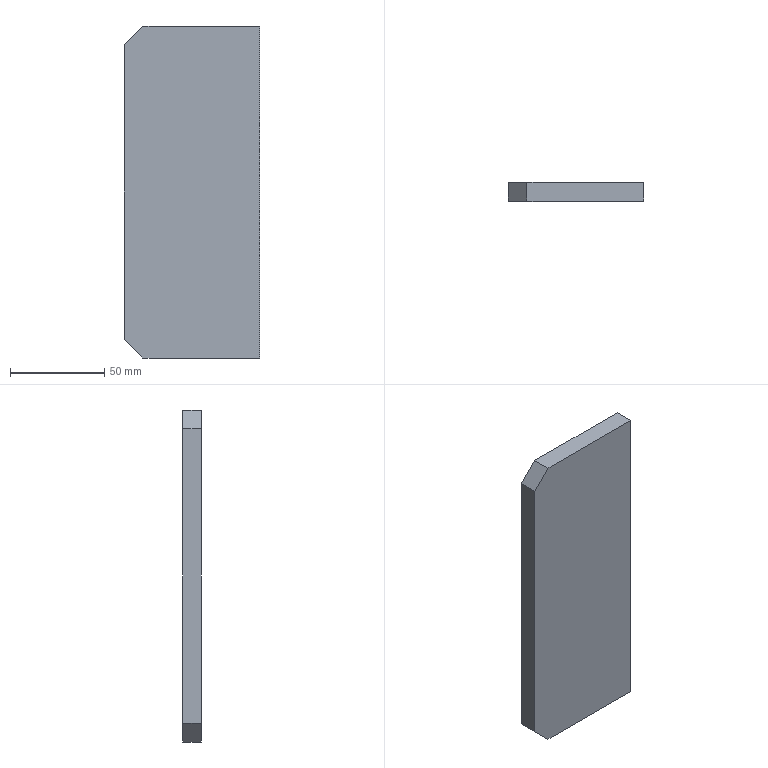Part | STEP file | 立柱填充筋Plate 200×150 | 1 solid | 8 faces | box 72 x 10 x 176 mm | volume 125720 mm3 | plane 8
STEP:
#1=CARTESIAN_POINT('',(0.,0.,0.));
#2=DIRECTION('',(0.,0.,1.));
#3=DIRECTION('',(1.,0.,0.));
#4=AXIS2_PLACEMENT_3D('',#1,#2,#3);
#5=CARTESIAN_POINT('',(72.,0.,88.));
#6=VERTEX_POINT('',#5);
#7=CARTESIAN_POINT('',(72.,0.,-88.));
#8=VERTEX_POINT('',#7);
#9=CARTESIAN_POINT('',(72.,0.,-88.));
#10=DIRECTION('',(0.,0.,-1.));
#11=VECTOR('',#10,1.);
#12=LINE('',#9,#11);
#13=CARTESIAN_POINT('',(72.,10.,-88.));
#14=DIRECTION('',(-1.,0.,0.));
#15=DIRECTION('',(0.,0.,1.));
#16=AXIS2_PLACEMENT_3D('',#13,#14,#15);
#17=PLANE('',#16);
#18=CARTESIAN_POINT('',(0.,-10.));
#19=DIRECTION('',(-1.,0.));
#20=VECTOR('',#19,1.);
#21=LINE('',#18,#20);
#22=(GEOMETRIC_REPRESENTATION_CONTEXT(2)PARAMETRIC_REPRESENTATION_CONTEXT()REPRESENTATION_CONTEXT('',''));
#23=DEFINITIONAL_REPRESENTATION('',(#21),#22);
#24=PCURVE('',#17,#23);
#25=CARTESIAN_POINT('',(0.,0.,0.));
#26=DIRECTION('',(0.,-1.,0.));
#27=DIRECTION('',(0.,0.,-1.));
#28=AXIS2_PLACEMENT_3D('',#25,#26,#27);
#29=PLANE('',#28);
#30=CARTESIAN_POINT('',(88.,72.));
#31=DIRECTION('',(1.,0.));
#32=VECTOR('',#31,1.);
#33=LINE('',#30,#32);
#34=(GEOMETRIC_REPRESENTATION_CONTEXT(2)PARAMETRIC_REPRESENTATION_CONTEXT()REPRESENTATION_CONTEXT('',''));
#35=DEFINITIONAL_REPRESENTATION('',(#33),#34);
#36=PCURVE('',#29,#35);
#37=SURFACE_CURVE('',#12,(#24,#36),.PCURVE_S1.);
#38=EDGE_CURVE('',#6,#8,#37,.T.);
#39=ORIENTED_EDGE('',*,*,#38,.T.);
#40=CARTESIAN_POINT('',(72.,10.,-88.));
#41=VERTEX_POINT('',#40);
#42=CARTESIAN_POINT('',(72.,10.,-88.));
#43=DIRECTION('',(0.,-1.,0.));
#44=VECTOR('',#43,1.);
#45=LINE('',#42,#44);
#46=CARTESIAN_POINT('',(0.,0.));
#47=DIRECTION('',(0.,-1.));
#48=VECTOR('',#47,1.);
#49=LINE('',#46,#48);
#50=(GEOMETRIC_REPRESENTATION_CONTEXT(2)PARAMETRIC_REPRESENTATION_CONTEXT()REPRESENTATION_CONTEXT('',''));
#51=DEFINITIONAL_REPRESENTATION('',(#49),#50);
#52=PCURVE('',#17,#51);
#53=CARTESIAN_POINT('',(0.,10.,-88.));
#54=DIRECTION('',(0.,0.,1.));
#55=DIRECTION('',(1.,0.,0.));
#56=AXIS2_PLACEMENT_3D('',#53,#54,#55);
#57=PLANE('',#56);
#58=CARTESIAN_POINT('',(72.,0.));
#59=DIRECTION('',(0.,-1.));
#60=VECTOR('',#59,1.);
#61=LINE('',#58,#60);
#62=(GEOMETRIC_REPRESENTATION_CONTEXT(2)PARAMETRIC_REPRESENTATION_CONTEXT()REPRESENTATION_CONTEXT('',''));
#63=DEFINITIONAL_REPRESENTATION('',(#61),#62);
#64=PCURVE('',#57,#63);
#65=SURFACE_CURVE('',#45,(#52,#64),.PCURVE_S1.);
#66=EDGE_CURVE('',#41,#8,#65,.T.);
#67=ORIENTED_EDGE('',*,*,#66,.F.);
#68=CARTESIAN_POINT('',(72.,10.,88.));
#69=VERTEX_POINT('',#68);
#70=CARTESIAN_POINT('',(72.,10.,-88.));
#71=DIRECTION('',(0.,0.,-1.));
#72=VECTOR('',#71,1.);
#73=LINE('',#70,#72);
#74=CARTESIAN_POINT('',(0.,0.));
#75=DIRECTION('',(-1.,0.));
#76=VECTOR('',#75,1.);
#77=LINE('',#74,#76);
#78=(GEOMETRIC_REPRESENTATION_CONTEXT(2)PARAMETRIC_REPRESENTATION_CONTEXT()REPRESENTATION_CONTEXT('',''));
#79=DEFINITIONAL_REPRESENTATION('',(#77),#78);
#80=PCURVE('',#17,#79);
#81=CARTESIAN_POINT('',(0.,10.,0.));
#82=DIRECTION('',(0.,-1.,0.));
#83=DIRECTION('',(0.,0.,-1.));
#84=AXIS2_PLACEMENT_3D('',#81,#82,#83);
#85=PLANE('',#84);
#86=CARTESIAN_POINT('',(88.,72.));
#87=DIRECTION('',(1.,0.));
#88=VECTOR('',#87,1.);
#89=LINE('',#86,#88);
#90=(GEOMETRIC_REPRESENTATION_CONTEXT(2)PARAMETRIC_REPRESENTATION_CONTEXT()REPRESENTATION_CONTEXT('',''));
#91=DEFINITIONAL_REPRESENTATION('',(#89),#90);
#92=PCURVE('',#85,#91);
#93=SURFACE_CURVE('',#73,(#80,#92),.PCURVE_S1.);
#94=EDGE_CURVE('',#69,#41,#93,.T.);
#95=ORIENTED_EDGE('',*,*,#94,.F.);
#96=CARTESIAN_POINT('',(72.,10.,88.));
#97=DIRECTION('',(0.,-1.,0.));
#98=VECTOR('',#97,1.);
#99=LINE('',#96,#98);
#100=CARTESIAN_POINT('',(176.,0.));
#101=DIRECTION('',(0.,-1.));
#102=VECTOR('',#101,1.);
#103=LINE('',#100,#102);
#104=(GEOMETRIC_REPRESENTATION_CONTEXT(2)PARAMETRIC_REPRESENTATION_CONTEXT()REPRESENTATION_CONTEXT('',''));
#105=DEFINITIONAL_REPRESENTATION('',(#103),#104);
#106=PCURVE('',#17,#105);
#107=CARTESIAN_POINT('',(72.,10.,88.));
#108=DIRECTION('',(0.,0.,-1.));
#109=DIRECTION('',(-1.,0.,0.));
#110=AXIS2_PLACEMENT_3D('',#107,#108,#109);
#111=PLANE('',#110);
#112=CARTESIAN_POINT('',(0.,0.));
#113=DIRECTION('',(0.,-1.));
#114=VECTOR('',#113,1.);
#115=LINE('',#112,#114);
#116=(GEOMETRIC_REPRESENTATION_CONTEXT(2)PARAMETRIC_REPRESENTATION_CONTEXT()REPRESENTATION_CONTEXT('',''));
#117=DEFINITIONAL_REPRESENTATION('',(#115),#116);
#118=PCURVE('',#111,#117);
#119=SURFACE_CURVE('',#99,(#106,#118),.PCURVE_S1.);
#120=EDGE_CURVE('',#69,#6,#119,.T.);
#121=ORIENTED_EDGE('',*,*,#120,.T.);
#122=EDGE_LOOP('',(#39,#67,#95,#121));
#123=FACE_BOUND('',#122,.T.);
#124=ADVANCED_FACE('',(#123),#17,.F.);
#125=CARTESIAN_POINT('',(10.,0.,-88.));
#126=VERTEX_POINT('',#125);
#127=CARTESIAN_POINT('',(0.,0.,-88.));
#128=DIRECTION('',(-1.,0.,0.));
#129=VECTOR('',#128,1.);
#130=LINE('',#127,#129);
#131=CARTESIAN_POINT('',(0.,-10.));
#132=DIRECTION('',(-1.,0.));
#133=VECTOR('',#132,1.);
#134=LINE('',#131,#133);
#135=(GEOMETRIC_REPRESENTATION_CONTEXT(2)PARAMETRIC_REPRESENTATION_CONTEXT()REPRESENTATION_CONTEXT('',''));
#136=DEFINITIONAL_REPRESENTATION('',(#134),#135);
#137=PCURVE('',#57,#136);
#138=CARTESIAN_POINT('',(88.,0.));
#139=DIRECTION('',(0.,-1.));
#140=VECTOR('',#139,1.);
#141=LINE('',#138,#140);
#142=(GEOMETRIC_REPRESENTATION_CONTEXT(2)PARAMETRIC_REPRESENTATION_CONTEXT()REPRESENTATION_CONTEXT('',''));
#143=DEFINITIONAL_REPRESENTATION('',(#141),#142);
#144=PCURVE('',#29,#143);
#145=SURFACE_CURVE('',#130,(#137,#144),.PCURVE_S1.);
#146=EDGE_CURVE('',#8,#126,#145,.T.);
#147=ORIENTED_EDGE('',*,*,#146,.T.);
#148=CARTESIAN_POINT('',(10.,10.,-88.));
#149=VERTEX_POINT('',#148);
#150=CARTESIAN_POINT('',(10.,10.,-88.));
#151=DIRECTION('',(0.,1.,0.));
#152=VECTOR('',#151,1.);
#153=LINE('',#150,#152);
#154=CARTESIAN_POINT('',(10.,0.));
#155=DIRECTION('',(0.,1.));
#156=VECTOR('',#155,1.);
#157=LINE('',#154,#156);
#158=(GEOMETRIC_REPRESENTATION_CONTEXT(2)PARAMETRIC_REPRESENTATION_CONTEXT()REPRESENTATION_CONTEXT('',''));
#159=DEFINITIONAL_REPRESENTATION('',(#157),#158);
#160=PCURVE('',#57,#159);
#161=CARTESIAN_POINT('',(0.,10.,-78.));
#162=DIRECTION('',(0.7071,0.,0.7071));
#163=DIRECTION('',(0.,-1.,0.));
#164=AXIS2_PLACEMENT_3D('',#161,#162,#163);
#165=PLANE('',#164);
#166=CARTESIAN_POINT('',(0.,14.142));
#167=DIRECTION('',(-1.,0.));
#168=VECTOR('',#167,1.);
#169=LINE('',#166,#168);
#170=(GEOMETRIC_REPRESENTATION_CONTEXT(2)PARAMETRIC_REPRESENTATION_CONTEXT()REPRESENTATION_CONTEXT('',''));
#171=DEFINITIONAL_REPRESENTATION('',(#169),#170);
#172=PCURVE('',#165,#171);
#173=SURFACE_CURVE('',#153,(#160,#172),.PCURVE_S1.);
#174=EDGE_CURVE('',#126,#149,#173,.T.);
#175=ORIENTED_EDGE('',*,*,#174,.T.);
#176=CARTESIAN_POINT('',(0.,10.,-88.));
#177=DIRECTION('',(-1.,0.,0.));
#178=VECTOR('',#177,1.);
#179=LINE('',#176,#178);
#180=CARTESIAN_POINT('',(0.,0.));
#181=DIRECTION('',(-1.,0.));
#182=VECTOR('',#181,1.);
#183=LINE('',#180,#182);
#184=(GEOMETRIC_REPRESENTATION_CONTEXT(2)PARAMETRIC_REPRESENTATION_CONTEXT()REPRESENTATION_CONTEXT('',''));
#185=DEFINITIONAL_REPRESENTATION('',(#183),#184);
#186=PCURVE('',#57,#185);
#187=CARTESIAN_POINT('',(88.,0.));
#188=DIRECTION('',(0.,-1.));
#189=VECTOR('',#188,1.);
#190=LINE('',#187,#189);
#191=(GEOMETRIC_REPRESENTATION_CONTEXT(2)PARAMETRIC_REPRESENTATION_CONTEXT()REPRESENTATION_CONTEXT('',''));
#192=DEFINITIONAL_REPRESENTATION('',(#190),#191);
#193=PCURVE('',#85,#192);
#194=SURFACE_CURVE('',#179,(#186,#193),.PCURVE_S1.);
#195=EDGE_CURVE('',#41,#149,#194,.T.);
#196=ORIENTED_EDGE('',*,*,#195,.F.);
#197=ORIENTED_EDGE('',*,*,#66,.T.);
#198=EDGE_LOOP('',(#147,#175,#196,#197));
#199=FACE_BOUND('',#198,.T.);
#200=ADVANCED_FACE('',(#199),#57,.F.);
#201=CARTESIAN_POINT('',(0.,0.,-78.));
#202=VERTEX_POINT('',#201);
#203=CARTESIAN_POINT('',(0.,0.,78.));
#204=VERTEX_POINT('',#203);
#205=CARTESIAN_POINT('',(0.,0.,88.));
#206=DIRECTION('',(0.,0.,1.));
#207=VECTOR('',#206,1.);
#208=LINE('',#205,#207);
#209=CARTESIAN_POINT('',(0.,10.,88.));
#210=DIRECTION('',(1.,0.,0.));
#211=DIRECTION('',(0.,0.,-1.));
#212=AXIS2_PLACEMENT_3D('',#209,#210,#211);
#213=PLANE('',#212);
#214=CARTESIAN_POINT('',(0.,-10.));
#215=DIRECTION('',(-1.,0.));
#216=VECTOR('',#215,1.);
#217=LINE('',#214,#216);
#218=(GEOMETRIC_REPRESENTATION_CONTEXT(2)PARAMETRIC_REPRESENTATION_CONTEXT()REPRESENTATION_CONTEXT('',''));
#219=DEFINITIONAL_REPRESENTATION('',(#217),#218);
#220=PCURVE('',#213,#219);
#221=CARTESIAN_POINT('',(-88.,0.));
#222=DIRECTION('',(-1.,0.));
#223=VECTOR('',#222,1.);
#224=LINE('',#221,#223);
#225=(GEOMETRIC_REPRESENTATION_CONTEXT(2)PARAMETRIC_REPRESENTATION_CONTEXT()REPRESENTATION_CONTEXT('',''));
#226=DEFINITIONAL_REPRESENTATION('',(#224),#225);
#227=PCURVE('',#29,#226);
#228=SURFACE_CURVE('',#208,(#220,#227),.PCURVE_S1.);
#229=EDGE_CURVE('',#202,#204,#228,.T.);
#230=ORIENTED_EDGE('',*,*,#229,.T.);
#231=CARTESIAN_POINT('',(0.,10.,78.));
#232=VERTEX_POINT('',#231);
#233=CARTESIAN_POINT('',(0.,10.,78.));
#234=DIRECTION('',(0.,1.,0.));
#235=VECTOR('',#234,1.);
#236=LINE('',#233,#235);
#237=CARTESIAN_POINT('',(10.,0.));
#238=DIRECTION('',(0.,1.));
#239=VECTOR('',#238,1.);
#240=LINE('',#237,#239);
#241=(GEOMETRIC_REPRESENTATION_CONTEXT(2)PARAMETRIC_REPRESENTATION_CONTEXT()REPRESENTATION_CONTEXT('',''));
#242=DEFINITIONAL_REPRESENTATION('',(#240),#241);
#243=PCURVE('',#213,#242);
#244=CARTESIAN_POINT('',(10.,10.,88.));
#245=DIRECTION('',(0.7071,0.,-0.7071));
#246=DIRECTION('',(0.,-1.,0.));
#247=AXIS2_PLACEMENT_3D('',#244,#245,#246);
#248=PLANE('',#247);
#249=CARTESIAN_POINT('',(0.,14.142));
#250=DIRECTION('',(-1.,0.));
#251=VECTOR('',#250,1.);
#252=LINE('',#249,#251);
#253=(GEOMETRIC_REPRESENTATION_CONTEXT(2)PARAMETRIC_REPRESENTATION_CONTEXT()REPRESENTATION_CONTEXT('',''));
#254=DEFINITIONAL_REPRESENTATION('',(#252),#253);
#255=PCURVE('',#248,#254);
#256=SURFACE_CURVE('',#236,(#243,#255),.PCURVE_S1.);
#257=EDGE_CURVE('',#204,#232,#256,.T.);
#258=ORIENTED_EDGE('',*,*,#257,.T.);
#259=CARTESIAN_POINT('',(0.,10.,-78.));
#260=VERTEX_POINT('',#259);
#261=CARTESIAN_POINT('',(0.,10.,88.));
#262=DIRECTION('',(0.,0.,1.));
#263=VECTOR('',#262,1.);
#264=LINE('',#261,#263);
#265=CARTESIAN_POINT('',(0.,0.));
#266=DIRECTION('',(-1.,0.));
#267=VECTOR('',#266,1.);
#268=LINE('',#265,#267);
#269=(GEOMETRIC_REPRESENTATION_CONTEXT(2)PARAMETRIC_REPRESENTATION_CONTEXT()REPRESENTATION_CONTEXT('',''));
#270=DEFINITIONAL_REPRESENTATION('',(#268),#269);
#271=PCURVE('',#213,#270);
#272=CARTESIAN_POINT('',(-88.,0.));
#273=DIRECTION('',(-1.,0.));
#274=VECTOR('',#273,1.);
#275=LINE('',#272,#274);
#276=(GEOMETRIC_REPRESENTATION_CONTEXT(2)PARAMETRIC_REPRESENTATION_CONTEXT()REPRESENTATION_CONTEXT('',''));
#277=DEFINITIONAL_REPRESENTATION('',(#275),#276);
#278=PCURVE('',#85,#277);
#279=SURFACE_CURVE('',#264,(#271,#278),.PCURVE_S1.);
#280=EDGE_CURVE('',#260,#232,#279,.T.);
#281=ORIENTED_EDGE('',*,*,#280,.F.);
#282=CARTESIAN_POINT('',(0.,10.,-78.));
#283=DIRECTION('',(0.,-1.,0.));
#284=VECTOR('',#283,1.);
#285=LINE('',#282,#284);
#286=CARTESIAN_POINT('',(166.,0.));
#287=DIRECTION('',(0.,-1.));
#288=VECTOR('',#287,1.);
#289=LINE('',#286,#288);
#290=(GEOMETRIC_REPRESENTATION_CONTEXT(2)PARAMETRIC_REPRESENTATION_CONTEXT()REPRESENTATION_CONTEXT('',''));
#291=DEFINITIONAL_REPRESENTATION('',(#289),#290);
#292=PCURVE('',#213,#291);
#293=CARTESIAN_POINT('',(0.,0.));
#294=DIRECTION('',(1.,0.));
#295=VECTOR('',#294,1.);
#296=LINE('',#293,#295);
#297=(GEOMETRIC_REPRESENTATION_CONTEXT(2)PARAMETRIC_REPRESENTATION_CONTEXT()REPRESENTATION_CONTEXT('',''));
#298=DEFINITIONAL_REPRESENTATION('',(#296),#297);
#299=PCURVE('',#165,#298);
#300=SURFACE_CURVE('',#285,(#292,#299),.PCURVE_S1.);
#301=EDGE_CURVE('',#260,#202,#300,.T.);
#302=ORIENTED_EDGE('',*,*,#301,.T.);
#303=EDGE_LOOP('',(#230,#258,#281,#302));
#304=FACE_BOUND('',#303,.T.);
#305=ADVANCED_FACE('',(#304),#213,.F.);
#306=CARTESIAN_POINT('',(10.,10.,88.));
#307=VERTEX_POINT('',#306);
#308=CARTESIAN_POINT('',(72.,10.,88.));
#309=DIRECTION('',(1.,0.,0.));
#310=VECTOR('',#309,1.);
#311=LINE('',#308,#310);
#312=CARTESIAN_POINT('',(0.,0.));
#313=DIRECTION('',(-1.,0.));
#314=VECTOR('',#313,1.);
#315=LINE('',#312,#314);
#316=(GEOMETRIC_REPRESENTATION_CONTEXT(2)PARAMETRIC_REPRESENTATION_CONTEXT()REPRESENTATION_CONTEXT('',''));
#317=DEFINITIONAL_REPRESENTATION('',(#315),#316);
#318=PCURVE('',#111,#317);
#319=CARTESIAN_POINT('',(-88.,72.));
#320=DIRECTION('',(0.,1.));
#321=VECTOR('',#320,1.);
#322=LINE('',#319,#321);
#323=(GEOMETRIC_REPRESENTATION_CONTEXT(2)PARAMETRIC_REPRESENTATION_CONTEXT()REPRESENTATION_CONTEXT('',''));
#324=DEFINITIONAL_REPRESENTATION('',(#322),#323);
#325=PCURVE('',#85,#324);
#326=SURFACE_CURVE('',#311,(#318,#325),.PCURVE_S1.);
#327=EDGE_CURVE('',#307,#69,#326,.T.);
#328=ORIENTED_EDGE('',*,*,#327,.F.);
#329=CARTESIAN_POINT('',(10.,0.,88.));
#330=VERTEX_POINT('',#329);
#331=CARTESIAN_POINT('',(10.,10.,88.));
#332=DIRECTION('',(0.,-1.,0.));
#333=VECTOR('',#332,1.);
#334=LINE('',#331,#333);
#335=CARTESIAN_POINT('',(62.,0.));
#336=DIRECTION('',(0.,-1.));
#337=VECTOR('',#336,1.);
#338=LINE('',#335,#337);
#339=(GEOMETRIC_REPRESENTATION_CONTEXT(2)PARAMETRIC_REPRESENTATION_CONTEXT()REPRESENTATION_CONTEXT('',''));
#340=DEFINITIONAL_REPRESENTATION('',(#338),#339);
#341=PCURVE('',#111,#340);
#342=CARTESIAN_POINT('',(0.,0.));
#343=DIRECTION('',(1.,0.));
#344=VECTOR('',#343,1.);
#345=LINE('',#342,#344);
#346=(GEOMETRIC_REPRESENTATION_CONTEXT(2)PARAMETRIC_REPRESENTATION_CONTEXT()REPRESENTATION_CONTEXT('',''));
#347=DEFINITIONAL_REPRESENTATION('',(#345),#346);
#348=PCURVE('',#248,#347);
#349=SURFACE_CURVE('',#334,(#341,#348),.PCURVE_S1.);
#350=EDGE_CURVE('',#307,#330,#349,.T.);
#351=ORIENTED_EDGE('',*,*,#350,.T.);
#352=CARTESIAN_POINT('',(72.,0.,88.));
#353=DIRECTION('',(1.,0.,0.));
#354=VECTOR('',#353,1.);
#355=LINE('',#352,#354);
#356=CARTESIAN_POINT('',(0.,-10.));
#357=DIRECTION('',(-1.,0.));
#358=VECTOR('',#357,1.);
#359=LINE('',#356,#358);
#360=(GEOMETRIC_REPRESENTATION_CONTEXT(2)PARAMETRIC_REPRESENTATION_CONTEXT()REPRESENTATION_CONTEXT('',''));
#361=DEFINITIONAL_REPRESENTATION('',(#359),#360);
#362=PCURVE('',#111,#361);
#363=CARTESIAN_POINT('',(-88.,72.));
#364=DIRECTION('',(0.,1.));
#365=VECTOR('',#364,1.);
#366=LINE('',#363,#365);
#367=(GEOMETRIC_REPRESENTATION_CONTEXT(2)PARAMETRIC_REPRESENTATION_CONTEXT()REPRESENTATION_CONTEXT('',''));
#368=DEFINITIONAL_REPRESENTATION('',(#366),#367);
#369=PCURVE('',#29,#368);
#370=SURFACE_CURVE('',#355,(#362,#369),.PCURVE_S1.);
#371=EDGE_CURVE('',#330,#6,#370,.T.);
#372=ORIENTED_EDGE('',*,*,#371,.T.);
#373=ORIENTED_EDGE('',*,*,#120,.F.);
#374=EDGE_LOOP('',(#328,#351,#372,#373));
#375=FACE_BOUND('',#374,.T.);
#376=ADVANCED_FACE('',(#375),#111,.F.);
#377=ORIENTED_EDGE('',*,*,#280,.T.);
#378=CARTESIAN_POINT('',(10.,10.,88.));
#379=DIRECTION('',(0.7071,0.,0.7071));
#380=VECTOR('',#379,1.);
#381=LINE('',#378,#380);
#382=CARTESIAN_POINT('',(-88.,10.));
#383=DIRECTION('',(-0.7071,0.7071));
#384=VECTOR('',#383,1.);
#385=LINE('',#382,#384);
#386=(GEOMETRIC_REPRESENTATION_CONTEXT(2)PARAMETRIC_REPRESENTATION_CONTEXT()REPRESENTATION_CONTEXT('',''));
#387=DEFINITIONAL_REPRESENTATION('',(#385),#386);
#388=PCURVE('',#85,#387);
#389=CARTESIAN_POINT('',(0.,0.));
#390=DIRECTION('',(0.,-1.));
#391=VECTOR('',#390,1.);
#392=LINE('',#389,#391);
#393=(GEOMETRIC_REPRESENTATION_CONTEXT(2)PARAMETRIC_REPRESENTATION_CONTEXT()REPRESENTATION_CONTEXT('',''));
#394=DEFINITIONAL_REPRESENTATION('',(#392),#393);
#395=PCURVE('',#248,#394);
#396=SURFACE_CURVE('',#381,(#388,#395),.PCURVE_S1.);
#397=EDGE_CURVE('',#232,#307,#396,.T.);
#398=ORIENTED_EDGE('',*,*,#397,.T.);
#399=ORIENTED_EDGE('',*,*,#327,.T.);
#400=ORIENTED_EDGE('',*,*,#94,.T.);
#401=ORIENTED_EDGE('',*,*,#195,.T.);
#402=CARTESIAN_POINT('',(0.,10.,-78.));
#403=DIRECTION('',(-0.7071,0.,0.7071));
#404=VECTOR('',#403,1.);
#405=LINE('',#402,#404);
#406=CARTESIAN_POINT('',(78.,0.));
#407=DIRECTION('',(-0.7071,-0.7071));
#408=VECTOR('',#407,1.);
#409=LINE('',#406,#408);
#410=(GEOMETRIC_REPRESENTATION_CONTEXT(2)PARAMETRIC_REPRESENTATION_CONTEXT()REPRESENTATION_CONTEXT('',''));
#411=DEFINITIONAL_REPRESENTATION('',(#409),#410);
#412=PCURVE('',#85,#411);
#413=CARTESIAN_POINT('',(0.,0.));
#414=DIRECTION('',(0.,-1.));
#415=VECTOR('',#414,1.);
#416=LINE('',#413,#415);
#417=(GEOMETRIC_REPRESENTATION_CONTEXT(2)PARAMETRIC_REPRESENTATION_CONTEXT()REPRESENTATION_CONTEXT('',''));
#418=DEFINITIONAL_REPRESENTATION('',(#416),#417);
#419=PCURVE('',#165,#418);
#420=SURFACE_CURVE('',#405,(#412,#419),.PCURVE_S1.);
#421=EDGE_CURVE('',#149,#260,#420,.T.);
#422=ORIENTED_EDGE('',*,*,#421,.T.);
#423=EDGE_LOOP('',(#377,#398,#399,#400,#401,#422));
#424=FACE_BOUND('',#423,.T.);
#425=ADVANCED_FACE('',(#424),#85,.F.);
#426=ORIENTED_EDGE('',*,*,#371,.F.);
#427=CARTESIAN_POINT('',(-39.,0.,39.));
#428=DIRECTION('',(-0.7071,0.,-0.7071));
#429=VECTOR('',#428,1.);
#430=LINE('',#427,#429);
#431=CARTESIAN_POINT('',(-39.,-39.));
#432=DIRECTION('',(0.7071,-0.7071));
#433=VECTOR('',#432,1.);
#434=LINE('',#431,#433);
#435=(GEOMETRIC_REPRESENTATION_CONTEXT(2)PARAMETRIC_REPRESENTATION_CONTEXT()REPRESENTATION_CONTEXT('',''));
#436=DEFINITIONAL_REPRESENTATION('',(#434),#435);
#437=PCURVE('',#29,#436);
#438=CARTESIAN_POINT('',(10.,69.296));
#439=DIRECTION('',(0.,1.));
#440=VECTOR('',#439,1.);
#441=LINE('',#438,#440);
#442=(GEOMETRIC_REPRESENTATION_CONTEXT(2)PARAMETRIC_REPRESENTATION_CONTEXT()REPRESENTATION_CONTEXT('',''));
#443=DEFINITIONAL_REPRESENTATION('',(#441),#442);
#444=PCURVE('',#248,#443);
#445=SURFACE_CURVE('',#430,(#437,#444),.PCURVE_S1.);
#446=EDGE_CURVE('',#330,#204,#445,.T.);
#447=ORIENTED_EDGE('',*,*,#446,.T.);
#448=ORIENTED_EDGE('',*,*,#229,.F.);
#449=CARTESIAN_POINT('',(-39.,0.,-39.));
#450=DIRECTION('',(0.7071,0.,-0.7071));
#451=VECTOR('',#450,1.);
#452=LINE('',#449,#451);
#453=CARTESIAN_POINT('',(39.,-39.));
#454=DIRECTION('',(0.7071,0.7071));
#455=VECTOR('',#454,1.);
#456=LINE('',#453,#455);
#457=(GEOMETRIC_REPRESENTATION_CONTEXT(2)PARAMETRIC_REPRESENTATION_CONTEXT()REPRESENTATION_CONTEXT('',''));
#458=DEFINITIONAL_REPRESENTATION('',(#456),#457);
#459=PCURVE('',#29,#458);
#460=CARTESIAN_POINT('',(10.,-55.154));
#461=DIRECTION('',(0.,1.));
#462=VECTOR('',#461,1.);
#463=LINE('',#460,#462);
#464=(GEOMETRIC_REPRESENTATION_CONTEXT(2)PARAMETRIC_REPRESENTATION_CONTEXT()REPRESENTATION_CONTEXT('',''));
#465=DEFINITIONAL_REPRESENTATION('',(#463),#464);
#466=PCURVE('',#165,#465);
#467=SURFACE_CURVE('',#452,(#459,#466),.PCURVE_S1.);
#468=EDGE_CURVE('',#202,#126,#467,.T.);
#469=ORIENTED_EDGE('',*,*,#468,.T.);
#470=ORIENTED_EDGE('',*,*,#146,.F.);
#471=ORIENTED_EDGE('',*,*,#38,.F.);
#472=EDGE_LOOP('',(#426,#447,#448,#469,#470,#471));
#473=FACE_BOUND('',#472,.T.);
#474=ADVANCED_FACE('',(#473),#29,.T.);
#475=ORIENTED_EDGE('',*,*,#397,.F.);
#476=ORIENTED_EDGE('',*,*,#257,.F.);
#477=ORIENTED_EDGE('',*,*,#446,.F.);
#478=ORIENTED_EDGE('',*,*,#350,.F.);
#479=EDGE_LOOP('',(#475,#476,#477,#478));
#480=FACE_BOUND('',#479,.T.);
#481=ADVANCED_FACE('',(#480),#248,.F.);
#482=ORIENTED_EDGE('',*,*,#421,.F.);
#483=ORIENTED_EDGE('',*,*,#174,.F.);
#484=ORIENTED_EDGE('',*,*,#468,.F.);
#485=ORIENTED_EDGE('',*,*,#301,.F.);
#486=EDGE_LOOP('',(#482,#483,#484,#485));
#487=FACE_BOUND('',#486,.T.);
#488=ADVANCED_FACE('',(#487),#165,.F.);
#489=CLOSED_SHELL('',(#124,#200,#305,#376,#425,#474,#481,#488));
#490=MANIFOLD_SOLID_BREP('',#489);
#491=(LENGTH_UNIT()NAMED_UNIT(*)SI_UNIT(.MILLI.,.METRE.));
#492=UNCERTAINTY_MEASURE_WITH_UNIT(LENGTH_MEASURE(0.0000001),#491,'','');
#493=(NAMED_UNIT(*)PLANE_ANGLE_UNIT()SI_UNIT($,.RADIAN.));
#494=(NAMED_UNIT(*)SI_UNIT($,.STERADIAN.)SOLID_ANGLE_UNIT());
#495=(GEOMETRIC_REPRESENTATION_CONTEXT(3)GLOBAL_UNCERTAINTY_ASSIGNED_CONTEXT((#492))GLOBAL_UNIT_ASSIGNED_CONTEXT((#491,#493,#494))REPRESENTATION_CONTEXT('',''));
#496=ADVANCED_BREP_SHAPE_REPRESENTATION('',(#4,#490),#495);